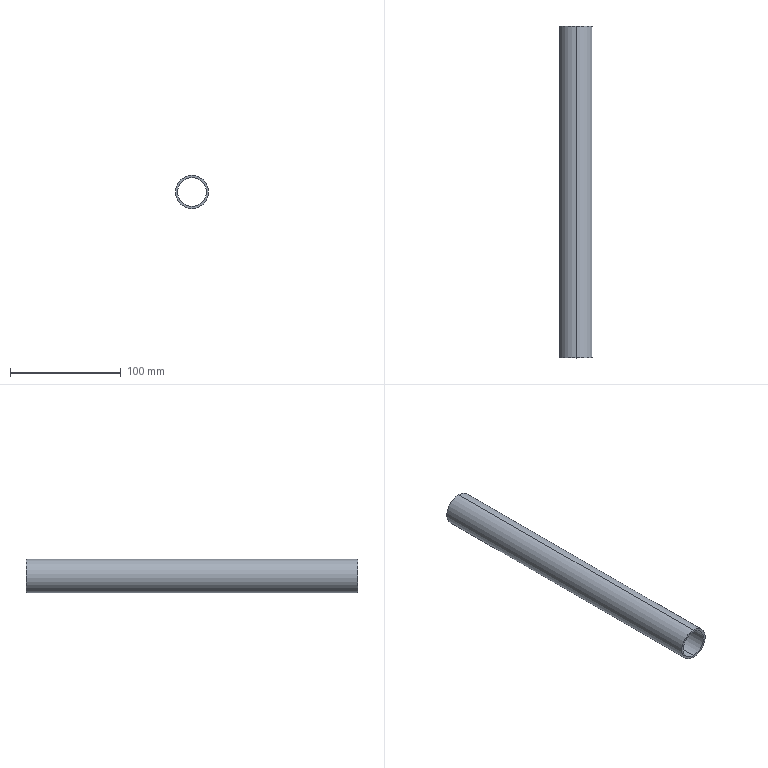Part | SolidWorks | features Sweep 1 | 1 solid | 6 faces | box 30 x 300 x 30 mm | volume 52779 mm3 | cylinder 4 | plane 2 | commonest cylinder face diameters 26 x2 30 x2
STEP:
#1=CARTESIAN_POINT('',(0.,0.,-13.));
#2=VERTEX_POINT('',#1);
#3=CARTESIAN_POINT('',(0.,0.,13.));
#4=VERTEX_POINT('',#3);
#5=CARTESIAN_POINT('',(0.,0.,0.));
#6=DIRECTION('',(0.,1.,0.));
#7=DIRECTION('',(0.,0.,1.));
#8=AXIS2_PLACEMENT_3D('',#5,#6,#7);
#9=CIRCLE('',#8,13.);
#10=EDGE_CURVE('',#2,#4,#9,.T.);
#11=ORIENTED_EDGE('',*,*,#10,.F.);
#12=CARTESIAN_POINT('',(0.,300.,-13.));
#13=VERTEX_POINT('',#12);
#14=CARTESIAN_POINT('',(0.,0.,-13.));
#15=DIRECTION('',(0.,1.,0.));
#16=VECTOR('',#15,1000.);
#17=LINE('',#14,#16);
#18=EDGE_CURVE('',#2,#13,#17,.T.);
#19=ORIENTED_EDGE('',*,*,#18,.T.);
#20=CARTESIAN_POINT('',(0.,300.,13.));
#21=VERTEX_POINT('',#20);
#22=CARTESIAN_POINT('',(0.,300.,0.));
#23=DIRECTION('',(0.,1.,0.));
#24=DIRECTION('',(0.,0.,1.));
#25=AXIS2_PLACEMENT_3D('',#22,#23,#24);
#26=CIRCLE('',#25,13.);
#27=EDGE_CURVE('',#13,#21,#26,.T.);
#28=ORIENTED_EDGE('',*,*,#27,.T.);
#29=CARTESIAN_POINT('',(0.,0.,13.));
#30=DIRECTION('',(0.,1.,0.));
#31=VECTOR('',#30,1000.);
#32=LINE('',#29,#31);
#33=EDGE_CURVE('',#4,#21,#32,.T.);
#34=ORIENTED_EDGE('',*,*,#33,.F.);
#35=EDGE_LOOP('',(#11,#19,#28,#34));
#36=FACE_OUTER_BOUND('',#35,.T.);
#37=CARTESIAN_POINT('',(0.,0.,0.));
#38=DIRECTION('',(0.,1.,0.));
#39=DIRECTION('',(0.,0.,1.));
#40=AXIS2_PLACEMENT_3D('',#37,#38,#39);
#41=CYLINDRICAL_SURFACE('',#40,13.);
#42=ADVANCED_FACE('',(#36),#41,.F.);
#43=CARTESIAN_POINT('',(0.,0.,15.));
#44=VERTEX_POINT('',#43);
#45=CARTESIAN_POINT('',(0.,0.,-15.));
#46=VERTEX_POINT('',#45);
#47=CARTESIAN_POINT('',(0.,0.,0.));
#48=DIRECTION('',(0.,1.,0.));
#49=DIRECTION('',(0.,0.,1.));
#50=AXIS2_PLACEMENT_3D('',#47,#48,#49);
#51=CIRCLE('',#50,15.);
#52=EDGE_CURVE('',#44,#46,#51,.T.);
#53=ORIENTED_EDGE('',*,*,#52,.T.);
#54=CARTESIAN_POINT('',(0.,300.,-15.));
#55=VERTEX_POINT('',#54);
#56=CARTESIAN_POINT('',(0.,0.,-15.));
#57=DIRECTION('',(0.,1.,0.));
#58=VECTOR('',#57,1000.);
#59=LINE('',#56,#58);
#60=EDGE_CURVE('',#46,#55,#59,.T.);
#61=ORIENTED_EDGE('',*,*,#60,.T.);
#62=CARTESIAN_POINT('',(0.,300.,15.));
#63=VERTEX_POINT('',#62);
#64=CARTESIAN_POINT('',(0.,300.,0.));
#65=DIRECTION('',(0.,1.,0.));
#66=DIRECTION('',(0.,0.,1.));
#67=AXIS2_PLACEMENT_3D('',#64,#65,#66);
#68=CIRCLE('',#67,15.);
#69=EDGE_CURVE('',#63,#55,#68,.T.);
#70=ORIENTED_EDGE('',*,*,#69,.F.);
#71=CARTESIAN_POINT('',(0.,0.,15.));
#72=DIRECTION('',(0.,1.,0.));
#73=VECTOR('',#72,1000.);
#74=LINE('',#71,#73);
#75=EDGE_CURVE('',#44,#63,#74,.T.);
#76=ORIENTED_EDGE('',*,*,#75,.F.);
#77=EDGE_LOOP('',(#53,#61,#70,#76));
#78=FACE_OUTER_BOUND('',#77,.T.);
#79=CARTESIAN_POINT('',(0.,0.,0.));
#80=DIRECTION('',(0.,1.,0.));
#81=DIRECTION('',(0.,0.,1.));
#82=AXIS2_PLACEMENT_3D('',#79,#80,#81);
#83=CYLINDRICAL_SURFACE('',#82,15.);
#84=ADVANCED_FACE('',(#78),#83,.T.);
#85=ORIENTED_EDGE('',*,*,#60,.F.);
#86=CARTESIAN_POINT('',(0.,0.,0.));
#87=DIRECTION('',(0.,1.,0.));
#88=DIRECTION('',(0.,0.,1.));
#89=AXIS2_PLACEMENT_3D('',#86,#87,#88);
#90=CIRCLE('',#89,15.);
#91=EDGE_CURVE('',#46,#44,#90,.T.);
#92=ORIENTED_EDGE('',*,*,#91,.T.);
#93=ORIENTED_EDGE('',*,*,#75,.T.);
#94=CARTESIAN_POINT('',(0.,300.,0.));
#95=DIRECTION('',(0.,1.,0.));
#96=DIRECTION('',(0.,0.,1.));
#97=AXIS2_PLACEMENT_3D('',#94,#95,#96);
#98=CIRCLE('',#97,15.);
#99=EDGE_CURVE('',#55,#63,#98,.T.);
#100=ORIENTED_EDGE('',*,*,#99,.F.);
#101=EDGE_LOOP('',(#85,#92,#93,#100));
#102=FACE_OUTER_BOUND('',#101,.T.);
#103=CARTESIAN_POINT('',(0.,0.,0.));
#104=DIRECTION('',(0.,1.,0.));
#105=DIRECTION('',(0.,0.,1.));
#106=AXIS2_PLACEMENT_3D('',#103,#104,#105);
#107=CYLINDRICAL_SURFACE('',#106,15.);
#108=ADVANCED_FACE('',(#102),#107,.T.);
#109=CARTESIAN_POINT('',(0.,300.,0.));
#110=DIRECTION('',(0.,1.,0.));
#111=DIRECTION('',(0.,0.,1.));
#112=AXIS2_PLACEMENT_3D('',#109,#110,#111);
#113=CIRCLE('',#112,13.);
#114=EDGE_CURVE('',#21,#13,#113,.T.);
#115=ORIENTED_EDGE('',*,*,#114,.F.);
#116=ORIENTED_EDGE('',*,*,#27,.F.);
#117=EDGE_LOOP('',(#115,#116));
#118=FACE_BOUND('',#117,.T.);
#119=ORIENTED_EDGE('',*,*,#69,.T.);
#120=ORIENTED_EDGE('',*,*,#99,.T.);
#121=EDGE_LOOP('',(#119,#120));
#122=FACE_OUTER_BOUND('',#121,.T.);
#123=CARTESIAN_POINT('',(0.,300.,0.));
#124=DIRECTION('',(0.,1.,0.));
#125=DIRECTION('',(0.,0.,1.));
#126=AXIS2_PLACEMENT_3D('',#123,#124,#125);
#127=PLANE('',#126);
#128=ADVANCED_FACE('',(#118,#122),#127,.T.);
#129=CARTESIAN_POINT('',(0.,0.,0.));
#130=DIRECTION('',(0.,1.,0.));
#131=DIRECTION('',(0.,0.,1.));
#132=AXIS2_PLACEMENT_3D('',#129,#130,#131);
#133=CIRCLE('',#132,13.);
#134=EDGE_CURVE('',#4,#2,#133,.T.);
#135=ORIENTED_EDGE('',*,*,#134,.T.);
#136=ORIENTED_EDGE('',*,*,#10,.T.);
#137=EDGE_LOOP('',(#135,#136));
#138=FACE_BOUND('',#137,.T.);
#139=ORIENTED_EDGE('',*,*,#52,.F.);
#140=ORIENTED_EDGE('',*,*,#91,.F.);
#141=EDGE_LOOP('',(#139,#140));
#142=FACE_OUTER_BOUND('',#141,.T.);
#143=CARTESIAN_POINT('',(0.,0.,0.));
#144=DIRECTION('',(0.,1.,0.));
#145=DIRECTION('',(0.,0.,1.));
#146=AXIS2_PLACEMENT_3D('',#143,#144,#145);
#147=PLANE('',#146);
#148=ADVANCED_FACE('',(#138,#142),#147,.F.);
#149=ORIENTED_EDGE('',*,*,#18,.F.);
#150=ORIENTED_EDGE('',*,*,#134,.F.);
#151=ORIENTED_EDGE('',*,*,#33,.T.);
#152=ORIENTED_EDGE('',*,*,#114,.T.);
#153=EDGE_LOOP('',(#149,#150,#151,#152));
#154=FACE_OUTER_BOUND('',#153,.T.);
#155=CARTESIAN_POINT('',(0.,0.,0.));
#156=DIRECTION('',(0.,1.,0.));
#157=DIRECTION('',(0.,0.,1.));
#158=AXIS2_PLACEMENT_3D('',#155,#156,#157);
#159=CYLINDRICAL_SURFACE('',#158,13.);
#160=ADVANCED_FACE('',(#154),#159,.F.);
#161=CLOSED_SHELL('',(#42,#84,#108,#128,#148,#160));
#162=MANIFOLD_SOLID_BREP('',#161);
#163=CARTESIAN_POINT('',(0.,0.,0.));
#164=DIRECTION('',(0.,0.,1.));
#165=DIRECTION('',(1.,0.,0.));
#166=AXIS2_PLACEMENT_3D('',#163,#164,#165);
#167=(LENGTH_UNIT()NAMED_UNIT(*)SI_UNIT(.MILLI.,.METRE.));
#168=UNCERTAINTY_MEASURE_WITH_UNIT(LENGTH_MEASURE(0.00001),#167,'','');
#169=(NAMED_UNIT(*)PLANE_ANGLE_UNIT()SI_UNIT($,.RADIAN.));
#170=(NAMED_UNIT(*)SI_UNIT($,.STERADIAN.)SOLID_ANGLE_UNIT());
#171=(GEOMETRIC_REPRESENTATION_CONTEXT(3)GLOBAL_UNCERTAINTY_ASSIGNED_CONTEXT((#168))GLOBAL_UNIT_ASSIGNED_CONTEXT((#167,#169,#170))REPRESENTATION_CONTEXT('',''));
#172=ADVANCED_BREP_SHAPE_REPRESENTATION('',(#162,#166),#171);